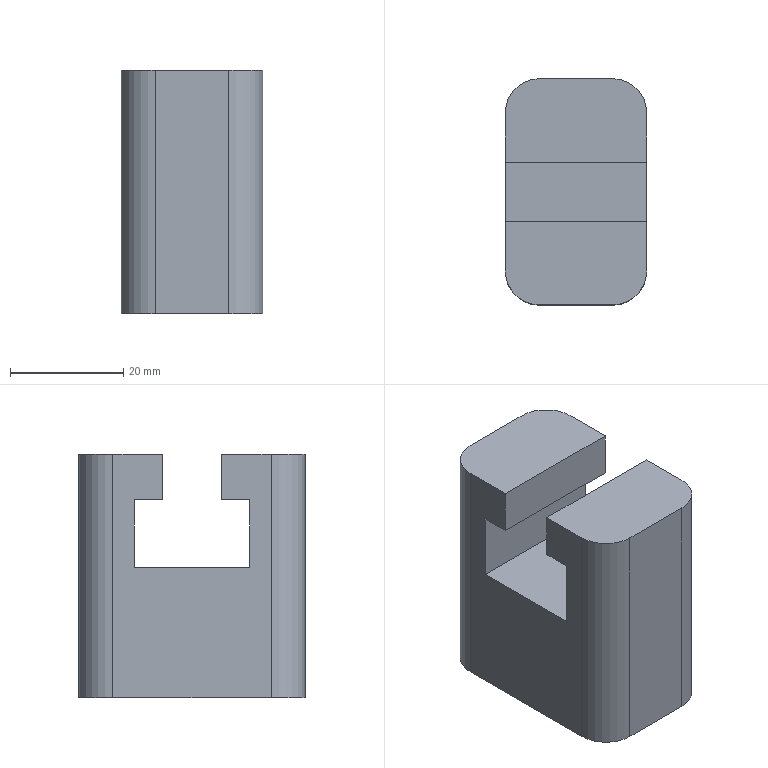Part | STEP file | solid 86 | 1 solid | 29 faces | box 25 x 40 x 43 mm | volume 32572 mm3 | plane 18 | cylinder 6 | other 4 | cone 1 | commonest cylinder face diameters 12 x4 6.7 x1 8 x1